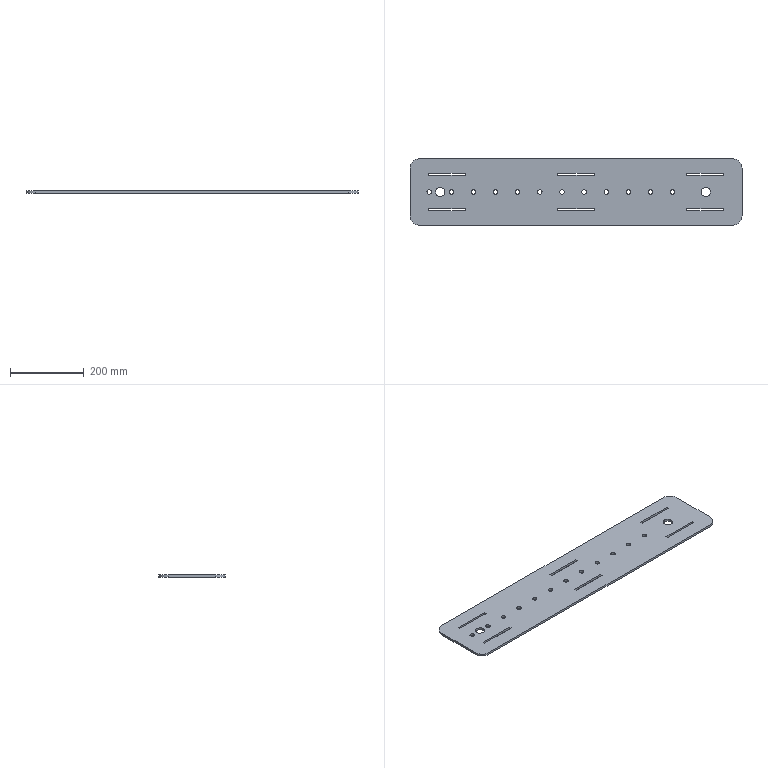Part | SolidWorks | features FlatPattern 1, SMBaseFlange 1, SheetMetal 1 | 1 solid | 62 faces | box 900 x 180 x 6 mm | volume 933147 mm3 | cylinder 32 | plane 30 | commonest cylinder face diameters 12 x24 25 x4 50 x4